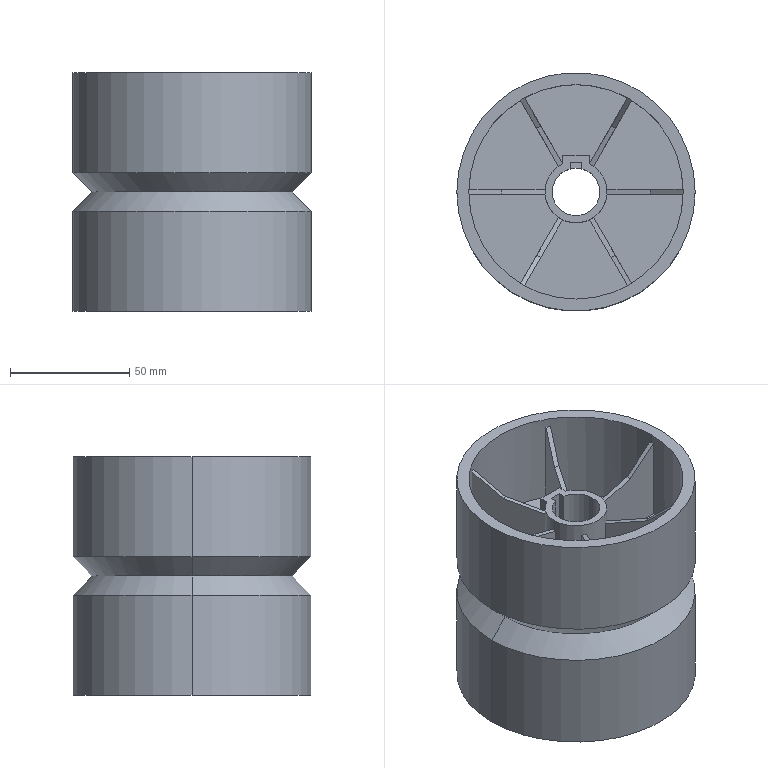Part | STEP file | 1 solid | 98 faces | box 100 x 100 x 100 mm | volume 282677 mm3 | plane 78 | cylinder 16 | cone 4 | commonest cylinder face diameters 26 x6 90 x4 100 x4 20 x2